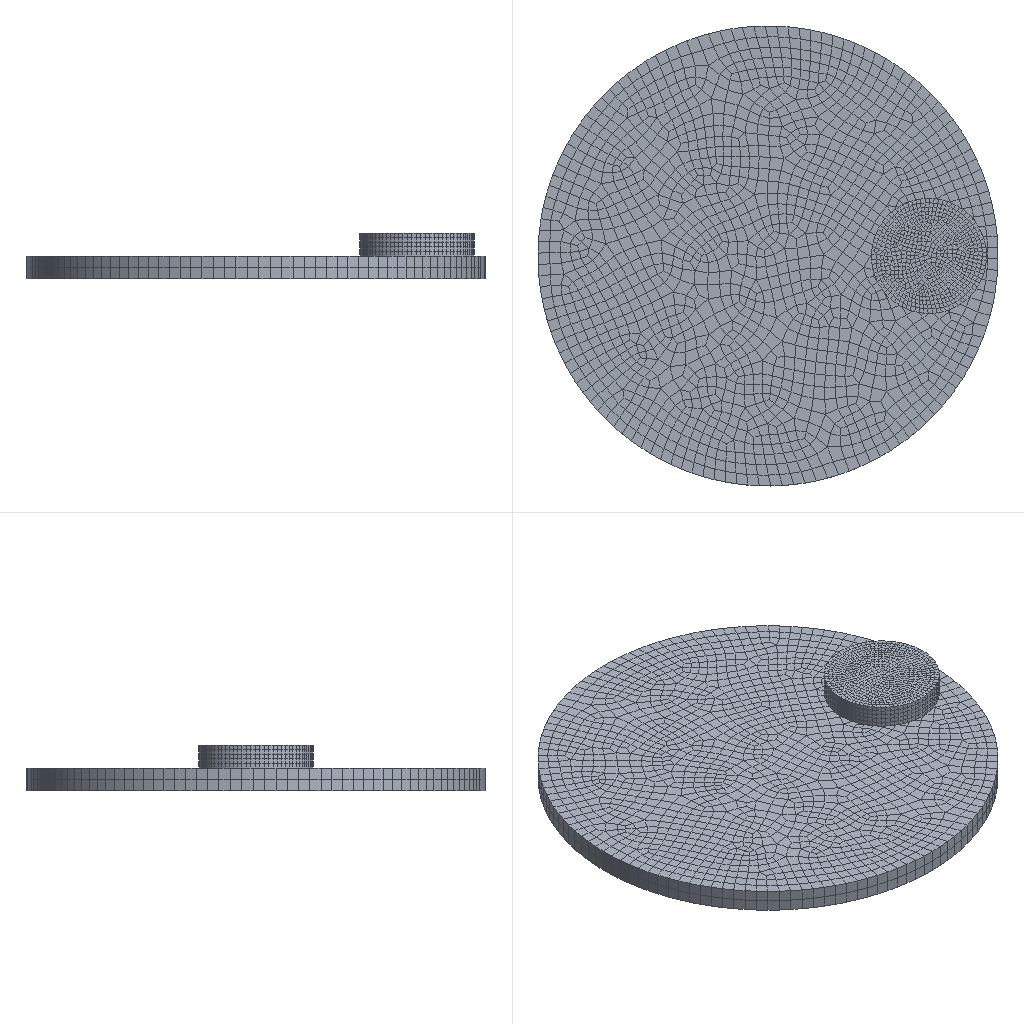Simulation study | abaqus
Set-up summary:
category,name,step,type,value,unit,region
solver,abaqus
solver,version,,,Abaqus/Standard 3DEXPERIENCE R2017x
units,not stated in the deck,,not stated
analysis,deck,,static,static
load_step,Step-1,Step-1,static
load_step,requested,,,1
mesh,nodes,,,9476
mesh,elements,,,6724
element_type,C3D8,,solid,6724
load,load commands in deck,,count,2
bc,support commands in deck,,count,6
material,MATERIAL-2,,in results
material,SMALL,,in results
check,setup vs results,,match,"per instance, exact: element labels, types and connectivity; labels of the nodes the elements use; coordinates of those nodes at SINGLE_PRECISION in 2 of 2 instance(s)"
Abaqus input file, long lists of numbers shortened:
*Heading
** Job name: Job-2 Model name: Model-1-no
** Generated by: Abaqus/CAE 2017
*Preprint, echo=NO, model=NO, history=NO, contact=NO
**
** PARTS
**
*Part, name=big
*Node
      1,   13.783,  -14.492,           0.
      2,   15.789,  -12.276,           0.
** (5026 more lines like these left out)
*Element, type=C3D8
   1, 2065, 2057, 1716, 1733,  389,  381,   40,   57
   2, 1717, 2135, 2123, 2059,   41,  459,  447,  383
** (3222 more lines like these left out)
*Node
   5029,           0.,  -1.2246468e-15,           2.
*Nset, nset=big-RefPt_, internal
5029,
*Nset, nset=Set-2, generate
    1,  5028,     1
*Elset, elset=Set-2, generate
    1,  3224,     1
** Section: Section-2
*Solid Section, elset=Set-2, material=Material-2
,
*End Part
**
*Part, name=small
*Node
      1,   4.428,  -2.323,           0.
      2,   4.736,  -1.602,           0.
** (4444 more lines like these left out)
*Element, type=C3D8
   1, 1356,  767,  814,  863,  615,   26,   73,  122
   2,  919,  813,  812,  918,  178,   72,   71,  177
** (3498 more lines like these left out)
*Node
   4447,           0.,  -3.061617e-16,           2.
*Nset, nset=small-RefPt_, internal
4447,
*Nset, nset=Set-1, generate
    1,  4446,     1
*Elset, elset=Set-1, generate
    1,  3500,     1
** Section: Section-1
*Solid Section, elset=Set-1, material=small
,
*End Part
**
**
** ASSEMBLY
**
*Assembly, name=Assembly
**
*Instance, name=big-1, part=big
*End Instance
**
*Instance, name=small-1, part=small
         14.,           0.,           2.
*End Instance
**
*Nset, nset=Set-3, instance=big-1
 5029,
*Nset, nset=Set-4, instance=small-1, generate
    1,  4447,     1
*Elset, elset=Set-4, instance=small-1, generate
    1,  3500,     1
*Nset, nset=Set-5, instance=small-1, generate
 3706,  4446,     1
*Elset, elset=Set-5, instance=small-1, generate
 2801,  3500,     1
*Nset, nset=Set-6, instance=big-1
 5029,
*Nset, nset=Set-8, instance=small-1, generate
   1,  741,    1
*Elset, elset=Set-8, instance=small-1, generate
   1,  700,    1
*Nset, nset=Set-9, instance=small-1, generate
 3706,  4446,     1
*Elset, elset=Set-9, instance=small-1, generate
 2801,  3500,     1
*Nset, nset=Set-11, instance=big-1
    1,    2,    3,    4,    5,    6,    7,    8,    9,   10,   11,   12,   13,   14,   15,   16
   17,   18,   19,   20,   21,   22,   23,   24,   25,   26,   27,   28,   29,   30,   31,   32
** (119 more lines like these left out)
*Elset, elset=Set-11, instance=big-1
    1,    2,    3,    4,    5,    6,    7,    8,    9,   10,   11,   12,   13,   14,   15,   16
   17,   18,   19,   20,   21,   22,   23,   24,   25,   26,   27,   28,   29,   30,   31,   32
** (107 more lines like these left out)
*Nset, nset=Set-12, instance=small-1, generate
 3706,  4446,     1
*Elset, elset=Set-12, instance=small-1, generate
 2801,  3500,     1
*Nset, nset=Set-14, instance=big-1
 5029,
*Nset, nset=Set-15, instance=big-1
 5029,
*Nset, nset=Set-16, instance=small-1, generate
   1,  741,    1
*Elset, elset=Set-16, instance=small-1, generate
   1,  700,    1
*Nset, nset=V, instance=small-1, generate
   1,  741,    1
*Elset, elset=V, instance=small-1, generate
   1,  700,    1
*Nset, nset=b_Set-1, instance=big-1, generate
    1,  5028,     1
*Elset, elset=b_Set-1, instance=big-1, generate
    1,  3224,     1
*Nset, nset=m_Set-13, instance=big-1
 5029,
*Nset, nset=_PickedSet7, internal, instance=big-1
 5029,
*Nset, nset=_PickedSet14, internal, instance=small-1, generate
    1,  4446,     1
*Elset, elset=_PickedSet14, internal, instance=small-1, generate
    1,  3500,     1
*Nset, nset=_PickedSet27, internal, instance=small-1, generate
    1,  4446,     1
*Elset, elset=_PickedSet27, internal, instance=small-1, generate
    1,  3500,     1
*Elset, elset=_Surf-3_S1, internal, instance=small-1, generate
 2801,  3500,     1
*Surface, type=ELEMENT, name=Surf-3
_Surf-3_S1, S1
*Elset, elset=_Surf-4_S2, internal, instance=big-1, generate
    1,  1612,     1
*Surface, type=ELEMENT, name=Surf-4
_Surf-4_S2, S2
*Elset, elset=_m_Surf-1_S1, internal, instance=big-1, generate
 1613,  3224,     1
*Surface, type=ELEMENT, name=m_Surf-1
_m_Surf-1_S1, S1
*Elset, elset=_s_Surf-1_S2, internal, instance=small-1, generate
   1,  700,    1
*Surface, type=ELEMENT, name=s_Surf-1
_s_Surf-1_S2, S2
*Elset, elset=_s_Surf-5_S4, internal, instance=big-1
    1,    9,   10,   13,   34,   40,   58,   78,   98,  112,  113,  148,  150,  157,  158,  160
  161,  171,  172,  173,  174,  175,  224,  250,  267,  270,  272,  274,  275,  307,  358,  512
** (6 more lines like these left out)
*Elset, elset=_s_Surf-5_S6, internal, instance=big-1
    2,    8,   11,   12,   32,   33,   36,   60,   94,  100,  115,  126,  128,  138,  151,  152
  159,  170,  225,  228,  234,  238,  242,  245,  246,  269,  393,  435,  475,  476,  506,  524
** (6 more lines like these left out)
*Elset, elset=_s_Surf-5_S5, internal, instance=big-1
  247, 1859
*Elset, elset=_s_Surf-5_S3, internal, instance=big-1
  519, 2131
*Elset, elset=_s_Surf-5_S2, internal, instance=big-1, generate
    1,  1612,     1
*Surface, type=ELEMENT, name=s_Surf-5
_s_Surf-5_S4, S4
_s_Surf-5_S6, S6
_s_Surf-5_S2, S2
_s_Surf-5_S5, S5
_s_Surf-5_S3, S3
** Constraint: Constraint-2
*Coupling, constraint name=Constraint-2, ref node=m_Set-13, surface=s_Surf-5
*Kinematic
*End Assembly
*Amplitude, name=Amp-1
         0.0166,     0.02325,          0.0333,     0.008997,            0.05,     0.00422,          0.0667,     0.01035
         0.0834,     0.008758,          0.1001,     0.01505,          0.1168,     0.01242,          0.1335,     0.02325
         0.1502,     0.01075,          0.1669,     0.01592,          0.1836,     0.0133,          0.2003,     0.003025
          0.217,     0.01473,          0.2337,     0.01624,          0.2504,     0.00215,          0.2671,     0.01959
         0.2838,     0.003185,          0.3005,     0.01513,          0.3172,     0.02213,          0.3339,     0.004379
         0.3506,     0.0199,          0.3673,     0.004379,           0.384,     0.007086,          0.4007,     0.0215
         0.4174,     0.007245,          0.4341,     0.01091,          0.4508,     0.009395,          0.4675,     0.008041
         0.4842,     0.01322,          0.5009,     0.003185,          0.5176,     0.02484,          0.5343,     0.01807
          0.551,     0.002787,          0.5677,     0.01481,          0.5844,      0.02094,          0.6011,     0.004857
         0.6178,     0.01919,          0.6345,     0.003424,          0.6512,     0.006768,          0.6679,     0.02142
         0.6846,     0.004459,          0.7013,     0.02341,           0.718,     0.00836,          0.7347,     0.007325
         0.7514,     0.01322,          0.7681,     0.002787,          0.7848,     0.02381,          0.8015,     0.01648
         0.8182,     0.001911,          0.8349,     0.01425,          0.8516,     0.02006,          0.8683,     0.01584
          0.885,     0.01768,          0.9017,     0.002787,          0.9184,     0.006051,          0.9351,      0.003662
         0.9518,     0.01919,          0.9685,     0.007643,          0.9852,     0.007086
**
** MATERIALS
**
*Material, name=Material-2
*Elastic
210000., 0.3
*Material, name=small
*Density
 6.89e-11,
*Elastic
 1.3, 0.3
**
** INTERACTION PROPERTIES
**
*Surface Interaction, name=IntProp-1
1.,
*Friction, slip tolerance=0.005
 0.25,
*Surface Behavior, pressure-overclosure=HARD
**
** INTERACTIONS
**
** Interaction: Int-1
*Contact Pair, interaction=IntProp-1, type=SURFACE TO SURFACE
s_Surf-1, m_Surf-1
** ----------------------------------------------------------------
**
** STEP: Step-1
**
*Step, name=Step-1, nlgeom=YES, inc=10000
*Static, stabilize=0.0002, allsdtol=0.05, continue=NO
0.001, 1., 1e-05, 1.
**
** BOUNDARY CONDITIONS
**
** Name: BC-2 Type: 对称/反对称/完全固定
*Boundary
Set-12, ENCASTRE
** Name: [REDACTED] : Displacement/rotation angle
*Boundary
Set-15, 1, 1
Set-15, 2, 2
Set-15, 4, 4
Set-15, 5, 5
Set-15, 6, 6, 12.57
*Adaptive Mesh Controls, name=Ada-1
0.5, 0.5
*Adaptive Mesh, elset=_PickedSet27, controls=Ada-1, frequency=1, mesh sweeps=2, op=NEW
**
** ADAPTIVE MESH CONSTRAINTS
**
** Name: Ada-Cons-2 Type: 速度/角速度
*Adaptive Mesh Constraint, user, type=VELOCITY
Set-16
**
** LOADS
**
** Name: Load-1   Type: Pressure
*Dsload, amplitude=Amp-1
Surf-4, P, 0.1
**
** OUTPUT REQUESTS
**
*Restart, write, frequency=0
**
** FIELD OUTPUT: F-Output-1
**
*Output, field
*Node Output
CF, COORD, RF, U, V
*Element Output, directions=YES
E, FV, IVOL, LE, MISES, PE, PEEQ, PEMAG, S, SDV, STH, SVOL, UVARM
*Contact Output
CDISP, CSTRESS
**
** HISTORY OUTPUT: H-Output-1
**
*Output, history
*Contact Output, master=m_Surf-1, slave=s_Surf-1
CAREA, CDISP
**
** HISTORY OUTPUT: V
**
*Element Output, elset=V
IVOL, VOL
*End Step
Results summary:
result,step,,partial,increments=154 time=0.6014/1.0
result,analysis,,,static
result,last_loadstep,,,1
result,primary field,,,U
result,reaction total,,FX,-0.0,model units
result,reaction total,,FY,0.0,model units
result,reaction total,,FZ,-0.6464,model units